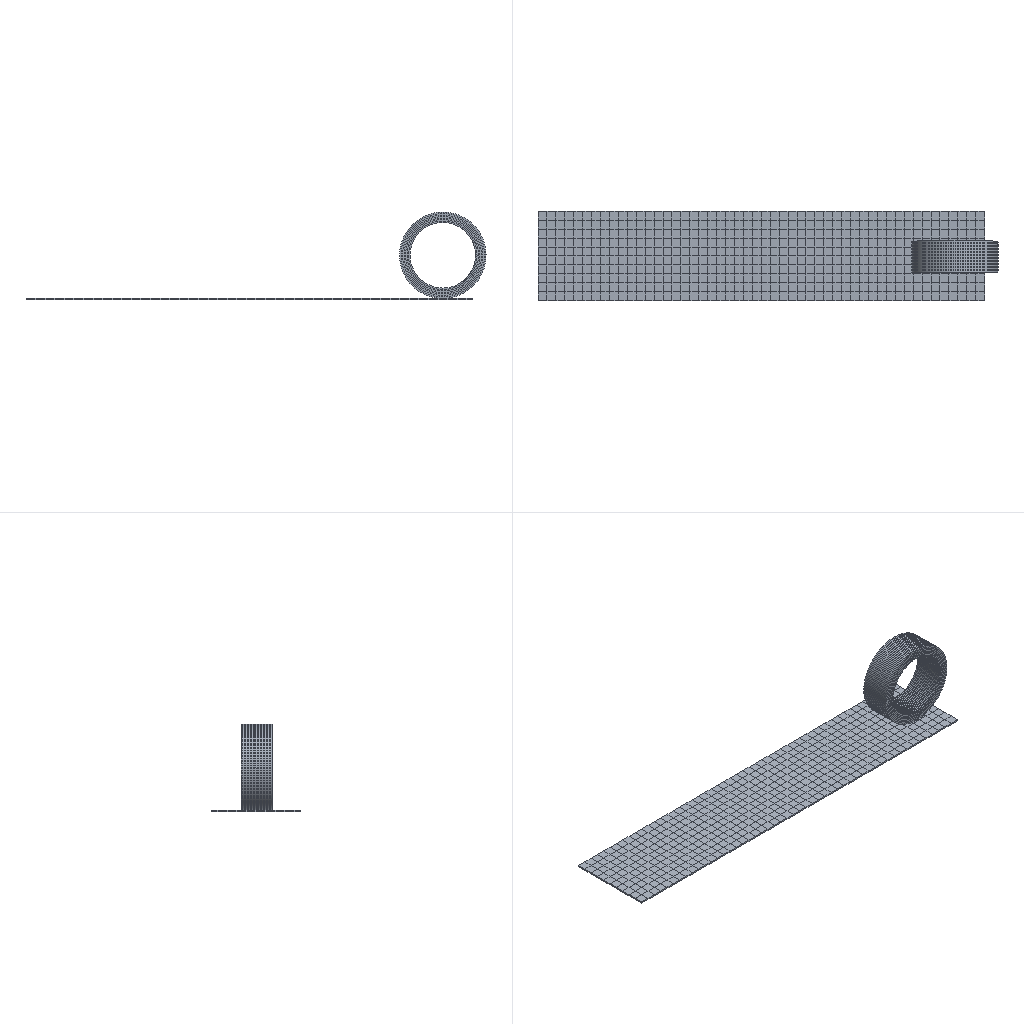Simulation study | abaqus
Set-up summary:
category,name,step,type,value,unit,region
solver,abaqus
solver,version,,,Abaqus/Standard 2020
units,not stated in the deck,,not stated
analysis,deck,,transient,transient
load_step,flat,flat,transient
load_step,load,load,transient
load_step,Step-3,Step-3,transient
load_step,Step-4,Step-4,transient
load_step,requested,,,4
mesh,nodes,,,26723
mesh,elements,,,18100
element_type,C3D8R,,solid,500
element_type,C3D8RH,,solid,17600
load,load commands in deck,,count,6
bc,support commands in deck,,count,50
material,BEAD,,in results
material,INSIDE,,in results
material,MATERIAL-9,,in results
material,PLY,,in results
material,RIMCONT,,in results
material,SANJIAO,,in results
material,SHOULDER,,in results
material,TREAD,,in results
material,UNDERTREAD,,in results
check,setup vs results,,match,"per instance, exact: element labels, types and connectivity; labels of the nodes the elements use; coordinates of those nodes at SINGLE_PRECISION in 1 of 2 instance(s)"
Abaqus input file, long lists of numbers shortened:
*Heading
** Job name: Job-3 Model name: fulltire-Copy2
** Generated by: Abaqus/CAE 2020
*Preprint, echo=NO, model=NO, history=NO, contact=NO
**
** PARTS
**
*Part, name=ground
*Node
      1,        3000.,           0.,          10.
      2,        3000.,         -60.,          10.
** (1120 more lines like these left out)
*Element, type=C3D8R
  1,   23,   24,   35,   34,    1,    2,   13,   12
  2,   24,   25,   36,   35,    2,    3,   14,   13
** (498 more lines like these left out)
*Node
   1123,        1500.,        -300.,          10.
*Nset, nset=ground-RefPt_, internal
1123,
*Nset, nset=Set-1, generate
    1,  1122,     1
*Elset, elset=Set-1, generate
   1,  500,    1
** Section: Section-13
*Solid Section, elset=Set-1, material=Material-9
,
*End Part
**
*Part, name=merge
*Node
      1,  -98.387,   196.774,         210.
      2,  -98.387,   196.774,           0.
** (25598 more lines like these left out)
*Element, type=C3D8RH
   1,    70,     5,  1522,    69,  6800,   508, 16178,  6799
   2,    68,  1522,  1497,    67,  1604, 16178, 16153,  1603
** (17598 more lines like these left out)
*Nset, nset=Set-2, generate
     1,  25600,      1
*Elset, elset=Set-2, generate
     1,  17600,      1
** Section: merge
*Solid Section, elset=Set-2, material=SANJIAO
,
*End Part
**
**
** ASSEMBLY
**
*Assembly, name=Assembly
**
*Instance, name=ground-1, part=ground
      -2750.,         300.,       -319.1
*End Instance
**
*Instance, name=merge-1, part=merge
         50.,         100.,        -19.1
         50.,         100.,        -19.1, 51.,         100.,        -19.1, 90.
*End Instance
**
*Node
      1,           0.,        -500.,        -350.
*Node
      2,           0.,           0.,           0.
*Node
      3,          50.,          -5.,  -19.1
*Nset, nset=Set-49
 2,
*Nset, nset=Set-50
 2,
*Nset, nset=Set-53
 2,
*Nset, nset=Set-54
 2,
*Nset, nset=Set-55, instance=ground-1
 1123,
*Nset, nset=Set-58, instance=ground-1
 1123,
*Nset, nset=Set-59
 2,
*Nset, nset=Set-61
 3,
*Nset, nset=Set-62
 3,
*Nset, nset=Set-63
 3,
*Nset, nset=Set-64, instance=ground-1
 1123,
*Nset, nset=Set-65
 3,
*Nset, nset=b_Set-56, instance=ground-1, generate
    1,  1122,     1
*Elset, elset=b_Set-56, instance=ground-1, generate
   1,  500,    1
*Nset, nset=m_Set-48
 2,
*Nset, nset=m_Set-60
 3,
*Nset, nset=_PickedSet100, internal, instance=ground-1
 1123,
*Elset, elset=_Surf-19_S3, internal, instance=merge-1
    30,    32,    34,    36,    97,   140,   142,   144,   146,   207,   250,   252,   254,   256,   317,   360
   362,   364,   366,   427,   470,   472,   474,   476,   537,   580,   582,   584,   586,   647,   690,   692
** (48 more lines like these left out)
*Elset, elset=_Surf-19_S5, internal, instance=merge-1
    38,    40,    42,    44,    46,    54,    55,    56,    58,    59,    61,    62,    64,    65,   148,   150
   152,   154,   156,   164,   165,   166,   168,   169,   171,   172,   174,   175,   258,   260,   262,   264
** (138 more lines like these left out)
*Surface, type=ELEMENT, name=Surf-19
_Surf-19_S3, S3
_Surf-19_S5, S5
*Elset, elset=_m_Surf-21_S6, internal, instance=merge-1
     2,     4,    29,    31,    33,    35,    37,    39,    41,    43,    45,    47,    48,   112,   114,   139
   141,   143,   145,   147,   149,   151,   153,   155,   157,   158,   222,   224,   249,   251,   253,   255
** (128 more lines like these left out)
*Elset, elset=_m_Surf-21_S4, internal, instance=merge-1
     3,    57,    60,    63,    93,    94,    95,    96,   113,   167,   170,   173,   203,   204,   205,   206
   223,   277,   280,   283,   313,   314,   315,   316,   333,   387,   390,   393,   423,   424,   425,   426
** (78 more lines like these left out)
*Surface, type=ELEMENT, name=m_Surf-21
_m_Surf-21_S6, S6
_m_Surf-21_S4, S4
*Elset, elset=_s_Surf-16_S3, internal, instance=ground-1, generate
   1,  500,    1
*Surface, type=ELEMENT, name=s_Surf-16
_s_Surf-16_S3, S3
*Elset, elset=_s_Surf-20_S6, internal, instance=merge-1, generate
     6,  17496,    110
*Elset, elset=_s_Surf-20_S5, internal, instance=merge-1
    16,    52,    88,    89,    90,   126,   162,   198,   199,   200,   236,   272,   308,   309,   310,   346
   382,   418,   419,   420,   456,   492,   528,   529,   530,   566,   602,   638,   639,   640,   676,   712
** (48 more lines like these left out)
*Elset, elset=_s_Surf-20_S3, internal, instance=merge-1
    24,    67,    71,    73,    75,    79,    81,    83,    85,    98,   101,   104,   107,   134,   177,   181
   183,   185,   189,   191,   193,   195,   208,   211,   214,   217,   244,   287,   291,   293,   295,   299
** (128 more lines like these left out)
*Elset, elset=_s_Surf-20_S4, internal, instance=merge-1
    53,    92,   163,   202,   273,   312,   383,   422,   493,   532,   603,   642,   713,   752,   823,   862
   933,   972,  1043,  1082,  1153,  1192,  1263,  1302,  1373,  1412,  1483,  1522,  1593,  1632,  1703,  1742
** (18 more lines like these left out)
*Surface, type=ELEMENT, name=s_Surf-20
_s_Surf-20_S6, S6
_s_Surf-20_S5, S5
_s_Surf-20_S4, S4
_s_Surf-20_S3, S3
*Elset, elset=_s_Surf-21_S3, internal, instance=ground-1, generate
   1,  500,    1
*Surface, type=ELEMENT, name=s_Surf-21
_s_Surf-21_S3, S3
** Constraint: Constraint-2
*Coupling, constraint name=Constraint-2, ref node=m_Set-60, surface=s_Surf-20
*Kinematic
** Constraint: Constraint-3
*Rigid Body, ref node=_PickedSet100, elset=b_Set-56, position=CENTER OF MASS
*End Assembly
*Amplitude, name=Amp-1
             0.,              0.,             0.5,              1.
*Amplitude, name=Amp-2
             0.,              0.,             0.2,              1.
**
** MATERIALS
**
**  THE PROPERTIES OF THE FOLLOWING MATERIALS MUST BE OBTAINED FROM THE
**  ORIGINAL MODEL DEFINITION
*Material, name=BEAD
*Density
 7.8e-09,
*Elastic
205500., 0.3
**  HMNAME MATS          2 inside     4
*Material, name=INSIDE
*Density
 1.5e-09,
*Hyperelastic, yeoh, moduli=LONG TERM
 0.45, -0.16, 0.079,    0.,    0.,    0.
*Viscoelastic, frequency=PRONY
 0.093,   0., 20.8
*Material, name=Material-9
*Density
 2e-09,
*Elastic
 1e+12, 0.2
**  HMNAME MATS          3 ply     5
*Material, name=PLY
*Density
 5.9e-09,
*Hyperelastic, marlow, moduli=LONG TERM
*Uniaxial Test Data
 -92.834, -0.09516
 -82.72, -0.08607
 -72.797, -0.07688
 -63.063, -0.06761
 -53.517, -0.05824
 -44.153, -0.04877
 -34.971, -0.03921
 -25.968, -0.02955
 -17.139, -0.0198
 -8.484, -0.00995
 -4.221, -0.004987
 -1.683,  -0.001998
 -0.8408, -0.0009995
       0.,         0.
   83.916,  0.001001
  167.664,   0.002002
  417.905, 0.005013
  831.642,  0.01005
  1646.73,  0.0202
  2445.52,  0.03045
  3228.25,  0.04081
  3995.16,  0.05127
  4746.49,  0.06184
  5482.48,  0.07251
  6203.34,  0.08329
  6909.32,  0.09417
  7600.63,   0.1052
*Viscoelastic, frequency=PRONY
 0.168,  0., 5.9
**  HMNAME MATS          4 rimcont     6
*Material, name=RIMCONT
*Density
 1.1e-09,
*Hyperelastic, neo hooke
 1.006, 0.02
**  HMNAME MATS          5 sanjiao     7
*Material, name=SANJIAO
*Density
 1.1e-09,
*Hyperelastic, neo hooke
 1.006, 0.02
**  HMNAME MATS          6 shoulder     8
*Material, name=SHOULDER
*Density
 1.1e-09,
*Hyperelastic, yeoh, moduli=LONG TERM
 0.47, -0.16, 0.084,    0.,    0.,    0.
*Viscoelastic, frequency=PRONY
 0.16,   0., 5.97
**  HMNAME MATS          7 tread     9
*Material, name=TREAD
*Density
 1.1e-09,
*Hyperelastic, yeoh, moduli=LONG TERM
 1.2, -1.2, 0.95,   0.,   0.,   0.
*Viscoelastic, frequency=PRONY
 0.125,    0., 6.512
**  HMNAME MATS          8 undertread    13
*Material, name=UNDERTREAD
*Density
 1.1e-09,
*Hyperelastic, neo hooke
 0.839, 0.024
**
** INTERACTION PROPERTIES
**
*Surface Interaction, name=IntProp-1
1.,
*Friction, slip tolerance=0.005
 0.8,
*Surface Behavior, pressure-overclosure=HARD
**
** BOUNDARY CONDITIONS
**
** Name: [REDACTED] : Displacement/rotation angle
*Boundary
Set-55, 1, 1
Set-55, 2, 2
Set-55, 3, 3
Set-55, 4, 4
Set-55, 5, 5
Set-55, 6, 6
**
** INTERACTIONS
**
** Interaction: Int-1
*Contact Pair, interaction=IntProp-1, type=SURFACE TO SURFACE
m_Surf-21, s_Surf-21
** ----------------------------------------------------------------
**
** STEP: flat
**
*Step, name=flat, nlgeom=YES, inc=1000
*Dynamic
0.01,0.2,2e-06
**
** LOADS
**
** Name: Load-1   Type: Pressure
*Dsload, amplitude=Amp-1
Surf-19, P, 0.01
**
** OUTPUT REQUESTS
**
*Restart, write, number interval=1, time marks=NO
**
** FIELD OUTPUT: F-Output-1
**
*Output, field, frequency=1
*Node Output
CF, RF, U
*Element Output, directions=YES
LE, PE, PEEQ, PEMAG, S
*Element Output, rebar, directions=YES
LE, PE, PEEQ, PEMAG, RBFOR, S
*Contact Output
CDISP, CSTRESS
**
** HISTORY OUTPUT: H-Output-1
**
*Output, history, variable=PRESELECT, frequency=1
*End Step
** ----------------------------------------------------------------
**
** STEP: load
**
*Step, name=load, nlgeom=YES, inc=1000
*Dynamic
0.01,0.2,2e-06
**
** BOUNDARY CONDITIONS
**
** Name: [REDACTED] : Velocity/Angular velocity
*Boundary, type=VELOCITY
Set-61, 1, 1
Set-61, 2, 2
Set-61, 3, 3
Set-61, 4, 4
Set-61, 5, 5
Set-61, 6, 6
** Name: [REDACTED] : Displacement/rotation angle
*Boundary, amplitude=Amp-2
Set-55, 1, 1
Set-55, 2, 2
Set-55, 3, 3, 5.
Set-55, 4, 4
Set-55, 5, 5
Set-55, 6, 6
**
** LOADS
**
** Name: Load-1   Type: Pressure
**
** OUTPUT REQUESTS
**
*Restart, write, frequency=0
**
** FIELD OUTPUT: F-Output-1
**
*Output, field, frequency=1
*Node Output
CF, RF, U
*Element Output, directions=YES
LE, PE, PEEQ, PEMAG, S
*Element Output, rebar, directions=YES
LE, PE, PEEQ, PEMAG, RBFOR, S
*Contact Output
CDISP, CSTRESS
**
** HISTORY OUTPUT: H-Output-1
**
*Output, history, variable=PRESELECT, frequency=1
*End Step
** ----------------------------------------------------------------
**
** STEP: Step-3
**
*Step, name=Step-3, nlgeom=YES, inc=100000
*Dynamic
0.001,0.4,4e-06
**
** BOUNDARY CONDITIONS
**
** Name: BC-4 Type: 速度/角速度
*Boundary, op=NEW, type=VELOCITY
Set-62, 2, 2
Set-62, 3, 3
Set-62, 4, 4
Set-62, 5, 5, -20.
Set-62, 6, 6
** Name: [REDACTED] : Velocity/Angular velocity
*Boundary, op=NEW, type=VELOCITY
Set-61, 2, 2
Set-61, 3, 3
Set-61, 4, 4
Set-61, 5, 5, -20.
Set-61, 6, 6
** Name: [REDACTED] : Displacement/rotation angle
*Boundary, op=NEW
Set-55, 1, 1
Set-55, 2, 2
Set-55, 3, 3, 5.
Set-55, 4, 4
Set-55, 5, 5
Set-55, 6, 6
**
** OUTPUT REQUESTS
**
*Restart, write, frequency=0
**
** FIELD OUTPUT: F-Output-1
**
*Output, field, frequency=2
*Node Output
CF, RF, U
*Element Output, directions=YES
LE, PE, PEEQ, PEMAG, S
*Element Output, rebar, directions=YES
LE, PE, PEEQ, PEMAG, RBFOR, S
*Contact Output
CDISP, CSTRESS
**
** HISTORY OUTPUT: H-Output-1
**
*Output, history, variable=PRESELECT, frequency=1
*End Step
** ----------------------------------------------------------------
**
** STEP: Step-4
**
*Step, name=Step-4, nlgeom=YES, inc=1000
*Dynamic
0.01,0.5,5e-06
**
** BOUNDARY CONDITIONS
**
** Name: BC-4 Type: 速度/角速度
*Boundary, op=NEW
** Name: BC-5 Type: 速度/角速度
*Boundary, op=NEW, type=VELOCITY
Set-65, 2, 2
Set-65, 3, 3
Set-65, 4, 4
Set-65, 5, 5
Set-65, 6, 6
** Name: [REDACTED] : Velocity/Angular velocity
*Boundary, op=NEW, type=VELOCITY
Set-61, 2, 2
Set-61, 3, 3
Set-61, 4, 4
Set-61, 5, 5
Set-61, 6, 6
** Name: [REDACTED] : Displacement/rotation angle
*Boundary, op=NEW
Set-55, 1, 1
Set-55, 2, 2
Set-55, 3, 3, 5.
Set-55, 4, 4
Set-55, 5, 5
Set-55, 6, 6
**
** OUTPUT REQUESTS
**
*Restart, write, frequency=0
**
** FIELD OUTPUT: F-Output-1
**
*Output, field, frequency=2
*Node Output
A, CF, RF, TF, U, V
*Element Output, directions=YES
E, LE, MISES, MISESMAX, PE, PEEQ, PEMAG, S, SF, SSAVG, TSHR
*Element Output, rebar, directions=YES
E, LE, MISES, MISESMAX, PE, PEEQ, PEMAG, RBFOR, S, SF, SSAVG, TSHR
*Contact Output
CDISP, CSTRESS
**
** HISTORY OUTPUT: H-Output-1
**
*Output, history, variable=PRESELECT, frequency=1
*End Step
Results summary:
result,step,,completed,increments=15 time=0.2/0.2
result,step,,completed,increments=12 time=0.2/0.2
result,step,,completed,increments=116 time=0.4/0.4
result,step,,completed,increments=19 time=0.5/0.5
result,analysis,,,transient
result,last_loadstep,,,4
result,primary field,,,U
result,reaction total,,FX,-110.126,model units
result,reaction total,,FY,-0.02912,model units
result,reaction total,,FZ,1.288,model units